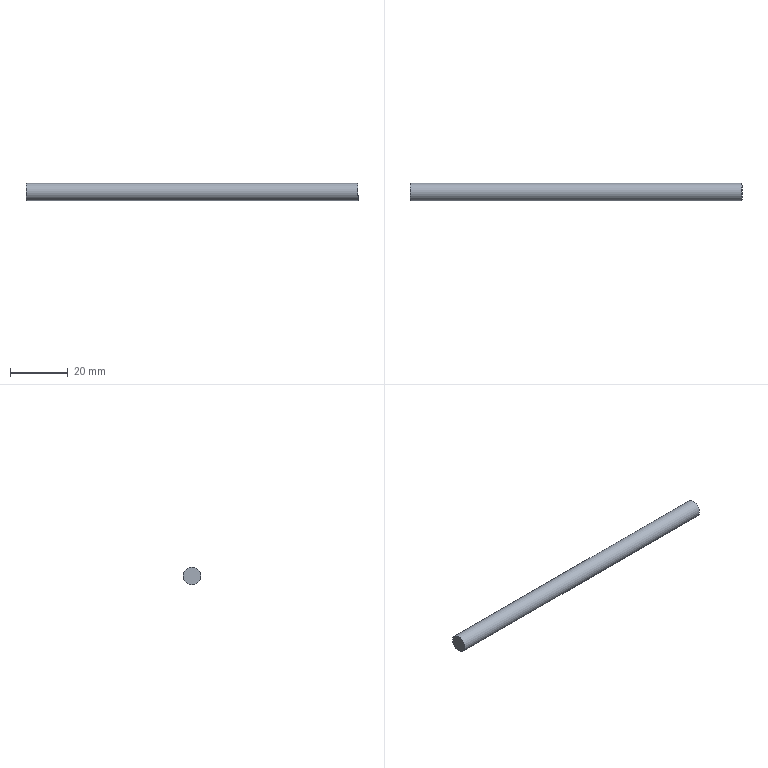Part | NX | features solid 2 | 1 solid | 3 faces | box 115 x 6 x 6 mm | volume 3252 mm3 | plane 2 | cylinder 1 | commonest cylinder face diameters 6 x1
STEP:
#1=CARTESIAN_POINT('',(-200.,-30.,103.));
#2=VERTEX_POINT('',#1);
#3=CARTESIAN_POINT('',(-200.,-30.,100.));
#4=DIRECTION('',(-1.,0.,0.));
#5=DIRECTION('',(0.,0.,1.));
#6=AXIS2_PLACEMENT_3D('',#3,#4,#5);
#7=CIRCLE('',#6,3.);
#8=EDGE_CURVE('',#2,#2,#7,.T.);
#9=ORIENTED_EDGE('',*,*,#8,.F.);
#10=EDGE_LOOP('',(#9));
#11=FACE_BOUND('',#10,.T.);
#12=CARTESIAN_POINT('',(-85.,-30.,103.));
#13=VERTEX_POINT('',#12);
#14=CARTESIAN_POINT('',(-85.,-30.,100.));
#15=DIRECTION('',(-1.,0.,0.));
#16=DIRECTION('',(0.,0.,1.));
#17=AXIS2_PLACEMENT_3D('',#14,#15,#16);
#18=CIRCLE('',#17,3.);
#19=EDGE_CURVE('',#13,#13,#18,.T.);
#20=ORIENTED_EDGE('',*,*,#19,.T.);
#21=EDGE_LOOP('',(#20));
#22=FACE_BOUND('',#21,.T.);
#23=CARTESIAN_POINT('',(-200.,-30.,100.));
#24=DIRECTION('',(1.,0.,0.));
#25=DIRECTION('',(0.,0.,-1.));
#26=AXIS2_PLACEMENT_3D('',#23,#24,#25);
#27=CYLINDRICAL_SURFACE('',#26,3.);
#28=ADVANCED_FACE('',(#11,#22),#27,.T.);
#29=ORIENTED_EDGE('',*,*,#8,.T.);
#30=EDGE_LOOP('',(#29));
#31=FACE_BOUND('',#30,.T.);
#32=CARTESIAN_POINT('',(-200.,-30.,100.));
#33=DIRECTION('',(-1.,0.,0.));
#34=DIRECTION('',(0.,0.,1.));
#35=AXIS2_PLACEMENT_3D('',#32,#33,#34);
#36=PLANE('',#35);
#37=ADVANCED_FACE('',(#31),#36,.T.);
#38=ORIENTED_EDGE('',*,*,#19,.F.);
#39=EDGE_LOOP('',(#38));
#40=FACE_BOUND('',#39,.T.);
#41=CARTESIAN_POINT('',(-85.,-30.,100.));
#42=DIRECTION('',(-1.,0.,0.));
#43=DIRECTION('',(0.,0.,1.));
#44=AXIS2_PLACEMENT_3D('',#41,#42,#43);
#45=PLANE('',#44);
#46=ADVANCED_FACE('',(#40),#45,.F.);
#47=CLOSED_SHELL('',(#28,#37,#46));
#48=MANIFOLD_SOLID_BREP('',#47);
#49=(LENGTH_UNIT()NAMED_UNIT(*)SI_UNIT(.MILLI.,.METRE.));
#50=UNCERTAINTY_MEASURE_WITH_UNIT(LENGTH_MEASURE(0.00001),#49,'','');
#51=(NAMED_UNIT(*)PLANE_ANGLE_UNIT()SI_UNIT($,.RADIAN.));
#52=(NAMED_UNIT(*)SI_UNIT($,.STERADIAN.)SOLID_ANGLE_UNIT());
#53=(GEOMETRIC_REPRESENTATION_CONTEXT(3)GLOBAL_UNCERTAINTY_ASSIGNED_CONTEXT((#50))GLOBAL_UNIT_ASSIGNED_CONTEXT((#49,#51,#52))REPRESENTATION_CONTEXT('',''));
#54=ADVANCED_BREP_SHAPE_REPRESENTATION('',(#48),#53);